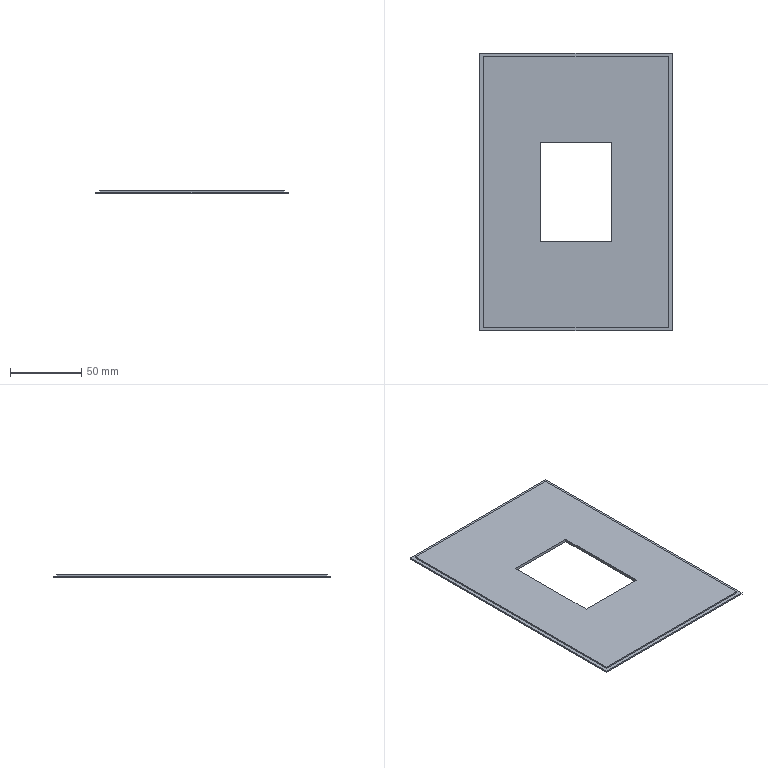Part | NX | 1 solid | 15 faces | box 135 x 195 x 2 mm | volume 44025 mm3 | plane 15
STEP:
#1=CARTESIAN_POINT('',(67.5,-97.5,1.));
#2=VERTEX_POINT('',#1);
#3=CARTESIAN_POINT('',(67.5,97.5,1.));
#4=VERTEX_POINT('',#3);
#5=CARTESIAN_POINT('',(67.5,97.5,1.));
#6=DIRECTION('',(0.,1.,0.));
#7=VECTOR('',#6,1000.);
#8=LINE('',#5,#7);
#9=EDGE_CURVE('',#2,#4,#8,.T.);
#10=ORIENTED_EDGE('',*,*,#9,.T.);
#11=CARTESIAN_POINT('',(-67.5,97.5,1.));
#12=VERTEX_POINT('',#11);
#13=CARTESIAN_POINT('',(-67.5,97.5,1.));
#14=DIRECTION('',(-1.,0.,0.));
#15=VECTOR('',#14,1000.);
#16=LINE('',#13,#15);
#17=EDGE_CURVE('',#4,#12,#16,.T.);
#18=ORIENTED_EDGE('',*,*,#17,.T.);
#19=CARTESIAN_POINT('',(-67.5,-97.5,1.));
#20=VERTEX_POINT('',#19);
#21=CARTESIAN_POINT('',(-67.5,97.5,1.));
#22=DIRECTION('',(0.,-1.,0.));
#23=VECTOR('',#22,1000.);
#24=LINE('',#21,#23);
#25=EDGE_CURVE('',#12,#20,#24,.T.);
#26=ORIENTED_EDGE('',*,*,#25,.T.);
#27=CARTESIAN_POINT('',(-67.5,-97.5,1.));
#28=DIRECTION('',(1.,0.,0.));
#29=VECTOR('',#28,1000.);
#30=LINE('',#27,#29);
#31=EDGE_CURVE('',#20,#2,#30,.T.);
#32=ORIENTED_EDGE('',*,*,#31,.T.);
#33=EDGE_LOOP('',(#10,#18,#26,#32));
#34=FACE_BOUND('',#33,.T.);
#35=CARTESIAN_POINT('',(65.,95.,1.));
#36=VERTEX_POINT('',#35);
#37=CARTESIAN_POINT('',(-65.,95.,1.));
#38=VERTEX_POINT('',#37);
#39=CARTESIAN_POINT('',(-65.,95.,1.));
#40=DIRECTION('',(-1.,0.,0.));
#41=VECTOR('',#40,1000.);
#42=LINE('',#39,#41);
#43=EDGE_CURVE('',#36,#38,#42,.T.);
#44=ORIENTED_EDGE('',*,*,#43,.F.);
#45=CARTESIAN_POINT('',(65.,-95.,1.));
#46=VERTEX_POINT('',#45);
#47=CARTESIAN_POINT('',(65.,95.,1.));
#48=DIRECTION('',(0.,1.,0.));
#49=VECTOR('',#48,1000.);
#50=LINE('',#47,#49);
#51=EDGE_CURVE('',#46,#36,#50,.T.);
#52=ORIENTED_EDGE('',*,*,#51,.F.);
#53=CARTESIAN_POINT('',(-65.,-95.,1.));
#54=VERTEX_POINT('',#53);
#55=CARTESIAN_POINT('',(-65.,-95.,1.));
#56=DIRECTION('',(1.,0.,0.));
#57=VECTOR('',#56,1000.);
#58=LINE('',#55,#57);
#59=EDGE_CURVE('',#54,#46,#58,.T.);
#60=ORIENTED_EDGE('',*,*,#59,.F.);
#61=CARTESIAN_POINT('',(-65.,95.,1.));
#62=DIRECTION('',(0.,-1.,0.));
#63=VECTOR('',#62,1000.);
#64=LINE('',#61,#63);
#65=EDGE_CURVE('',#38,#54,#64,.T.);
#66=ORIENTED_EDGE('',*,*,#65,.F.);
#67=EDGE_LOOP('',(#44,#52,#60,#66));
#68=FACE_BOUND('',#67,.T.);
#69=CARTESIAN_POINT('',(0.,0.,1.));
#70=DIRECTION('',(0.,0.,1.));
#71=DIRECTION('',(1.,0.,0.));
#72=AXIS2_PLACEMENT_3D('',#69,#70,#71);
#73=PLANE('',#72);
#74=ADVANCED_FACE('',(#34,#68),#73,.T.);
#75=CARTESIAN_POINT('',(67.5,-97.5,0.));
#76=VERTEX_POINT('',#75);
#77=CARTESIAN_POINT('',(67.5,97.5,0.));
#78=VERTEX_POINT('',#77);
#79=CARTESIAN_POINT('',(67.5,97.5,0.));
#80=DIRECTION('',(0.,1.,0.));
#81=VECTOR('',#80,1000.);
#82=LINE('',#79,#81);
#83=EDGE_CURVE('',#76,#78,#82,.T.);
#84=ORIENTED_EDGE('',*,*,#83,.T.);
#85=CARTESIAN_POINT('',(67.5,97.5,1.));
#86=DIRECTION('',(0.,0.,-1.));
#87=VECTOR('',#86,1000.);
#88=LINE('',#85,#87);
#89=EDGE_CURVE('',#4,#78,#88,.T.);
#90=ORIENTED_EDGE('',*,*,#89,.F.);
#91=ORIENTED_EDGE('',*,*,#9,.F.);
#92=CARTESIAN_POINT('',(67.5,-97.5,1.));
#93=DIRECTION('',(0.,0.,-1.));
#94=VECTOR('',#93,1000.);
#95=LINE('',#92,#94);
#96=EDGE_CURVE('',#2,#76,#95,.T.);
#97=ORIENTED_EDGE('',*,*,#96,.T.);
#98=EDGE_LOOP('',(#84,#90,#91,#97));
#99=FACE_BOUND('',#98,.T.);
#100=CARTESIAN_POINT('',(67.5,97.5,1.));
#101=DIRECTION('',(-1.,0.,0.));
#102=DIRECTION('',(0.,-1.,0.));
#103=AXIS2_PLACEMENT_3D('',#100,#101,#102);
#104=PLANE('',#103);
#105=ADVANCED_FACE('',(#99),#104,.F.);
#106=CARTESIAN_POINT('',(-67.5,97.5,0.));
#107=VERTEX_POINT('',#106);
#108=CARTESIAN_POINT('',(-67.5,97.5,0.));
#109=DIRECTION('',(-1.,0.,0.));
#110=VECTOR('',#109,1000.);
#111=LINE('',#108,#110);
#112=EDGE_CURVE('',#78,#107,#111,.T.);
#113=ORIENTED_EDGE('',*,*,#112,.T.);
#114=CARTESIAN_POINT('',(-67.5,97.5,1.));
#115=DIRECTION('',(0.,0.,-1.));
#116=VECTOR('',#115,1000.);
#117=LINE('',#114,#116);
#118=EDGE_CURVE('',#12,#107,#117,.T.);
#119=ORIENTED_EDGE('',*,*,#118,.F.);
#120=ORIENTED_EDGE('',*,*,#17,.F.);
#121=ORIENTED_EDGE('',*,*,#89,.T.);
#122=EDGE_LOOP('',(#113,#119,#120,#121));
#123=FACE_BOUND('',#122,.T.);
#124=CARTESIAN_POINT('',(-67.5,97.5,1.));
#125=DIRECTION('',(0.,-1.,0.));
#126=DIRECTION('',(0.,0.,-1.));
#127=AXIS2_PLACEMENT_3D('',#124,#125,#126);
#128=PLANE('',#127);
#129=ADVANCED_FACE('',(#123),#128,.F.);
#130=CARTESIAN_POINT('',(-67.5,-97.5,0.));
#131=VERTEX_POINT('',#130);
#132=CARTESIAN_POINT('',(-67.5,97.5,0.));
#133=DIRECTION('',(0.,-1.,0.));
#134=VECTOR('',#133,1000.);
#135=LINE('',#132,#134);
#136=EDGE_CURVE('',#107,#131,#135,.T.);
#137=ORIENTED_EDGE('',*,*,#136,.T.);
#138=CARTESIAN_POINT('',(-67.5,-97.5,1.));
#139=DIRECTION('',(0.,0.,-1.));
#140=VECTOR('',#139,1000.);
#141=LINE('',#138,#140);
#142=EDGE_CURVE('',#20,#131,#141,.T.);
#143=ORIENTED_EDGE('',*,*,#142,.F.);
#144=ORIENTED_EDGE('',*,*,#25,.F.);
#145=ORIENTED_EDGE('',*,*,#118,.T.);
#146=EDGE_LOOP('',(#137,#143,#144,#145));
#147=FACE_BOUND('',#146,.T.);
#148=CARTESIAN_POINT('',(-67.5,97.5,1.));
#149=DIRECTION('',(1.,0.,0.));
#150=DIRECTION('',(0.,1.,0.));
#151=AXIS2_PLACEMENT_3D('',#148,#149,#150);
#152=PLANE('',#151);
#153=ADVANCED_FACE('',(#147),#152,.F.);
#154=CARTESIAN_POINT('',(-67.5,-97.5,0.));
#155=DIRECTION('',(1.,0.,0.));
#156=VECTOR('',#155,1000.);
#157=LINE('',#154,#156);
#158=EDGE_CURVE('',#131,#76,#157,.T.);
#159=ORIENTED_EDGE('',*,*,#158,.T.);
#160=ORIENTED_EDGE('',*,*,#96,.F.);
#161=ORIENTED_EDGE('',*,*,#31,.F.);
#162=ORIENTED_EDGE('',*,*,#142,.T.);
#163=EDGE_LOOP('',(#159,#160,#161,#162));
#164=FACE_BOUND('',#163,.T.);
#165=CARTESIAN_POINT('',(-67.5,-97.5,1.));
#166=DIRECTION('',(0.,1.,0.));
#167=DIRECTION('',(0.,0.,1.));
#168=AXIS2_PLACEMENT_3D('',#165,#166,#167);
#169=PLANE('',#168);
#170=ADVANCED_FACE('',(#164),#169,.F.);
#171=CARTESIAN_POINT('',(-25.,-35.,0.));
#172=VERTEX_POINT('',#171);
#173=CARTESIAN_POINT('',(25.,-35.,0.));
#174=VERTEX_POINT('',#173);
#175=CARTESIAN_POINT('',(0.,-35.,0.));
#176=DIRECTION('',(1.,0.,0.));
#177=VECTOR('',#176,1000.);
#178=LINE('',#175,#177);
#179=EDGE_CURVE('',#172,#174,#178,.T.);
#180=ORIENTED_EDGE('',*,*,#179,.T.);
#181=CARTESIAN_POINT('',(25.,35.,0.));
#182=VERTEX_POINT('',#181);
#183=CARTESIAN_POINT('',(25.,0.,0.));
#184=DIRECTION('',(0.,1.,0.));
#185=VECTOR('',#184,1000.);
#186=LINE('',#183,#185);
#187=EDGE_CURVE('',#174,#182,#186,.T.);
#188=ORIENTED_EDGE('',*,*,#187,.T.);
#189=CARTESIAN_POINT('',(-25.,35.,0.));
#190=VERTEX_POINT('',#189);
#191=CARTESIAN_POINT('',(0.,35.,0.));
#192=DIRECTION('',(-1.,0.,0.));
#193=VECTOR('',#192,1000.);
#194=LINE('',#191,#193);
#195=EDGE_CURVE('',#182,#190,#194,.T.);
#196=ORIENTED_EDGE('',*,*,#195,.T.);
#197=CARTESIAN_POINT('',(-25.,0.,0.));
#198=DIRECTION('',(0.,-1.,0.));
#199=VECTOR('',#198,1000.);
#200=LINE('',#197,#199);
#201=EDGE_CURVE('',#190,#172,#200,.T.);
#202=ORIENTED_EDGE('',*,*,#201,.T.);
#203=EDGE_LOOP('',(#180,#188,#196,#202));
#204=FACE_BOUND('',#203,.T.);
#205=ORIENTED_EDGE('',*,*,#83,.F.);
#206=ORIENTED_EDGE('',*,*,#158,.F.);
#207=ORIENTED_EDGE('',*,*,#136,.F.);
#208=ORIENTED_EDGE('',*,*,#112,.F.);
#209=EDGE_LOOP('',(#205,#206,#207,#208));
#210=FACE_BOUND('',#209,.T.);
#211=CARTESIAN_POINT('',(0.,0.,0.));
#212=DIRECTION('',(0.,0.,1.));
#213=DIRECTION('',(1.,0.,0.));
#214=AXIS2_PLACEMENT_3D('',#211,#212,#213);
#215=PLANE('',#214);
#216=ADVANCED_FACE('',(#204,#210),#215,.F.);
#217=ORIENTED_EDGE('',*,*,#51,.T.);
#218=CARTESIAN_POINT('',(65.,95.,2.));
#219=VERTEX_POINT('',#218);
#220=CARTESIAN_POINT('',(65.,95.,2.));
#221=DIRECTION('',(0.,0.,-1.));
#222=VECTOR('',#221,1000.);
#223=LINE('',#220,#222);
#224=EDGE_CURVE('',#219,#36,#223,.T.);
#225=ORIENTED_EDGE('',*,*,#224,.F.);
#226=CARTESIAN_POINT('',(65.,-95.,2.));
#227=VERTEX_POINT('',#226);
#228=CARTESIAN_POINT('',(65.,95.,2.));
#229=DIRECTION('',(0.,1.,0.));
#230=VECTOR('',#229,1000.);
#231=LINE('',#228,#230);
#232=EDGE_CURVE('',#227,#219,#231,.T.);
#233=ORIENTED_EDGE('',*,*,#232,.F.);
#234=CARTESIAN_POINT('',(65.,-95.,2.));
#235=DIRECTION('',(0.,0.,-1.));
#236=VECTOR('',#235,1000.);
#237=LINE('',#234,#236);
#238=EDGE_CURVE('',#227,#46,#237,.T.);
#239=ORIENTED_EDGE('',*,*,#238,.T.);
#240=EDGE_LOOP('',(#217,#225,#233,#239));
#241=FACE_BOUND('',#240,.T.);
#242=CARTESIAN_POINT('',(65.,95.,2.));
#243=DIRECTION('',(-1.,0.,0.));
#244=DIRECTION('',(0.,-1.,0.));
#245=AXIS2_PLACEMENT_3D('',#242,#243,#244);
#246=PLANE('',#245);
#247=ADVANCED_FACE('',(#241),#246,.F.);
#248=ORIENTED_EDGE('',*,*,#43,.T.);
#249=CARTESIAN_POINT('',(-65.,95.,2.));
#250=VERTEX_POINT('',#249);
#251=CARTESIAN_POINT('',(-65.,95.,2.));
#252=DIRECTION('',(0.,0.,-1.));
#253=VECTOR('',#252,1000.);
#254=LINE('',#251,#253);
#255=EDGE_CURVE('',#250,#38,#254,.T.);
#256=ORIENTED_EDGE('',*,*,#255,.F.);
#257=CARTESIAN_POINT('',(-65.,95.,2.));
#258=DIRECTION('',(-1.,0.,0.));
#259=VECTOR('',#258,1000.);
#260=LINE('',#257,#259);
#261=EDGE_CURVE('',#219,#250,#260,.T.);
#262=ORIENTED_EDGE('',*,*,#261,.F.);
#263=ORIENTED_EDGE('',*,*,#224,.T.);
#264=EDGE_LOOP('',(#248,#256,#262,#263));
#265=FACE_BOUND('',#264,.T.);
#266=CARTESIAN_POINT('',(-65.,95.,2.));
#267=DIRECTION('',(0.,-1.,0.));
#268=DIRECTION('',(0.,0.,-1.));
#269=AXIS2_PLACEMENT_3D('',#266,#267,#268);
#270=PLANE('',#269);
#271=ADVANCED_FACE('',(#265),#270,.F.);
#272=ORIENTED_EDGE('',*,*,#65,.T.);
#273=CARTESIAN_POINT('',(-65.,-95.,2.));
#274=VERTEX_POINT('',#273);
#275=CARTESIAN_POINT('',(-65.,-95.,2.));
#276=DIRECTION('',(0.,0.,-1.));
#277=VECTOR('',#276,1000.);
#278=LINE('',#275,#277);
#279=EDGE_CURVE('',#274,#54,#278,.T.);
#280=ORIENTED_EDGE('',*,*,#279,.F.);
#281=CARTESIAN_POINT('',(-65.,95.,2.));
#282=DIRECTION('',(0.,-1.,0.));
#283=VECTOR('',#282,1000.);
#284=LINE('',#281,#283);
#285=EDGE_CURVE('',#250,#274,#284,.T.);
#286=ORIENTED_EDGE('',*,*,#285,.F.);
#287=ORIENTED_EDGE('',*,*,#255,.T.);
#288=EDGE_LOOP('',(#272,#280,#286,#287));
#289=FACE_BOUND('',#288,.T.);
#290=CARTESIAN_POINT('',(-65.,95.,2.));
#291=DIRECTION('',(1.,0.,0.));
#292=DIRECTION('',(0.,1.,0.));
#293=AXIS2_PLACEMENT_3D('',#290,#291,#292);
#294=PLANE('',#293);
#295=ADVANCED_FACE('',(#289),#294,.F.);
#296=ORIENTED_EDGE('',*,*,#59,.T.);
#297=ORIENTED_EDGE('',*,*,#238,.F.);
#298=CARTESIAN_POINT('',(-65.,-95.,2.));
#299=DIRECTION('',(1.,0.,0.));
#300=VECTOR('',#299,1000.);
#301=LINE('',#298,#300);
#302=EDGE_CURVE('',#274,#227,#301,.T.);
#303=ORIENTED_EDGE('',*,*,#302,.F.);
#304=ORIENTED_EDGE('',*,*,#279,.T.);
#305=EDGE_LOOP('',(#296,#297,#303,#304));
#306=FACE_BOUND('',#305,.T.);
#307=CARTESIAN_POINT('',(-65.,-95.,2.));
#308=DIRECTION('',(0.,1.,0.));
#309=DIRECTION('',(0.,0.,1.));
#310=AXIS2_PLACEMENT_3D('',#307,#308,#309);
#311=PLANE('',#310);
#312=ADVANCED_FACE('',(#306),#311,.F.);
#313=CARTESIAN_POINT('',(25.,-35.,2.));
#314=VERTEX_POINT('',#313);
#315=CARTESIAN_POINT('',(25.,35.,2.));
#316=VERTEX_POINT('',#315);
#317=CARTESIAN_POINT('',(25.,35.,2.));
#318=DIRECTION('',(0.,1.,0.));
#319=VECTOR('',#318,1000.);
#320=LINE('',#317,#319);
#321=EDGE_CURVE('',#314,#316,#320,.T.);
#322=ORIENTED_EDGE('',*,*,#321,.F.);
#323=CARTESIAN_POINT('',(-25.,-35.,2.));
#324=VERTEX_POINT('',#323);
#325=CARTESIAN_POINT('',(-25.,-35.,2.));
#326=DIRECTION('',(1.,0.,0.));
#327=VECTOR('',#326,1000.);
#328=LINE('',#325,#327);
#329=EDGE_CURVE('',#324,#314,#328,.T.);
#330=ORIENTED_EDGE('',*,*,#329,.F.);
#331=CARTESIAN_POINT('',(-25.,35.,2.));
#332=VERTEX_POINT('',#331);
#333=CARTESIAN_POINT('',(-25.,35.,2.));
#334=DIRECTION('',(0.,-1.,0.));
#335=VECTOR('',#334,1000.);
#336=LINE('',#333,#335);
#337=EDGE_CURVE('',#332,#324,#336,.T.);
#338=ORIENTED_EDGE('',*,*,#337,.F.);
#339=CARTESIAN_POINT('',(-25.,35.,2.));
#340=DIRECTION('',(-1.,0.,0.));
#341=VECTOR('',#340,1000.);
#342=LINE('',#339,#341);
#343=EDGE_CURVE('',#316,#332,#342,.T.);
#344=ORIENTED_EDGE('',*,*,#343,.F.);
#345=EDGE_LOOP('',(#322,#330,#338,#344));
#346=FACE_BOUND('',#345,.T.);
#347=ORIENTED_EDGE('',*,*,#232,.T.);
#348=ORIENTED_EDGE('',*,*,#261,.T.);
#349=ORIENTED_EDGE('',*,*,#285,.T.);
#350=ORIENTED_EDGE('',*,*,#302,.T.);
#351=EDGE_LOOP('',(#347,#348,#349,#350));
#352=FACE_BOUND('',#351,.T.);
#353=CARTESIAN_POINT('',(0.,0.,2.));
#354=DIRECTION('',(0.,0.,1.));
#355=DIRECTION('',(1.,0.,0.));
#356=AXIS2_PLACEMENT_3D('',#353,#354,#355);
#357=PLANE('',#356);
#358=ADVANCED_FACE('',(#346,#352),#357,.T.);
#359=CARTESIAN_POINT('',(25.,-35.,-1.));
#360=DIRECTION('',(0.,0.,1.));
#361=VECTOR('',#360,1000.);
#362=LINE('',#359,#361);
#363=EDGE_CURVE('',#174,#314,#362,.T.);
#364=ORIENTED_EDGE('',*,*,#363,.T.);
#365=ORIENTED_EDGE('',*,*,#321,.T.);
#366=CARTESIAN_POINT('',(25.,35.,-1.));
#367=DIRECTION('',(0.,0.,1.));
#368=VECTOR('',#367,1000.);
#369=LINE('',#366,#368);
#370=EDGE_CURVE('',#182,#316,#369,.T.);
#371=ORIENTED_EDGE('',*,*,#370,.F.);
#372=ORIENTED_EDGE('',*,*,#187,.F.);
#373=EDGE_LOOP('',(#364,#365,#371,#372));
#374=FACE_BOUND('',#373,.T.);
#375=CARTESIAN_POINT('',(25.,35.,-1.));
#376=DIRECTION('',(1.,0.,0.));
#377=DIRECTION('',(0.,1.,0.));
#378=AXIS2_PLACEMENT_3D('',#375,#376,#377);
#379=PLANE('',#378);
#380=ADVANCED_FACE('',(#374),#379,.F.);
#381=CARTESIAN_POINT('',(-25.,-35.,-1.));
#382=DIRECTION('',(0.,0.,1.));
#383=VECTOR('',#382,1000.);
#384=LINE('',#381,#383);
#385=EDGE_CURVE('',#172,#324,#384,.T.);
#386=ORIENTED_EDGE('',*,*,#385,.T.);
#387=ORIENTED_EDGE('',*,*,#329,.T.);
#388=ORIENTED_EDGE('',*,*,#363,.F.);
#389=ORIENTED_EDGE('',*,*,#179,.F.);
#390=EDGE_LOOP('',(#386,#387,#388,#389));
#391=FACE_BOUND('',#390,.T.);
#392=CARTESIAN_POINT('',(-25.,-35.,-1.));
#393=DIRECTION('',(0.,-1.,0.));
#394=DIRECTION('',(0.,0.,-1.));
#395=AXIS2_PLACEMENT_3D('',#392,#393,#394);
#396=PLANE('',#395);
#397=ADVANCED_FACE('',(#391),#396,.F.);
#398=CARTESIAN_POINT('',(-25.,35.,-1.));
#399=DIRECTION('',(0.,0.,1.));
#400=VECTOR('',#399,1000.);
#401=LINE('',#398,#400);
#402=EDGE_CURVE('',#190,#332,#401,.T.);
#403=ORIENTED_EDGE('',*,*,#402,.T.);
#404=ORIENTED_EDGE('',*,*,#337,.T.);
#405=ORIENTED_EDGE('',*,*,#385,.F.);
#406=ORIENTED_EDGE('',*,*,#201,.F.);
#407=EDGE_LOOP('',(#403,#404,#405,#406));
#408=FACE_BOUND('',#407,.T.);
#409=CARTESIAN_POINT('',(-25.,35.,-1.));
#410=DIRECTION('',(-1.,0.,0.));
#411=DIRECTION('',(0.,-1.,0.));
#412=AXIS2_PLACEMENT_3D('',#409,#410,#411);
#413=PLANE('',#412);
#414=ADVANCED_FACE('',(#408),#413,.F.);
#415=ORIENTED_EDGE('',*,*,#370,.T.);
#416=ORIENTED_EDGE('',*,*,#343,.T.);
#417=ORIENTED_EDGE('',*,*,#402,.F.);
#418=ORIENTED_EDGE('',*,*,#195,.F.);
#419=EDGE_LOOP('',(#415,#416,#417,#418));
#420=FACE_BOUND('',#419,.T.);
#421=CARTESIAN_POINT('',(-25.,35.,-1.));
#422=DIRECTION('',(0.,1.,0.));
#423=DIRECTION('',(0.,0.,1.));
#424=AXIS2_PLACEMENT_3D('',#421,#422,#423);
#425=PLANE('',#424);
#426=ADVANCED_FACE('',(#420),#425,.F.);
#427=CLOSED_SHELL('',(#74,#105,#129,#153,#170,#216,#247,#271,#295,#312,#358,#380,#397,#414,#426));
#428=MANIFOLD_SOLID_BREP('',#427);
#429=(LENGTH_UNIT()NAMED_UNIT(*)SI_UNIT(.MILLI.,.METRE.));
#430=UNCERTAINTY_MEASURE_WITH_UNIT(LENGTH_MEASURE(0.00001),#429,'','');
#431=(NAMED_UNIT(*)PLANE_ANGLE_UNIT()SI_UNIT($,.RADIAN.));
#432=(NAMED_UNIT(*)SI_UNIT($,.STERADIAN.)SOLID_ANGLE_UNIT());
#433=(GEOMETRIC_REPRESENTATION_CONTEXT(3)GLOBAL_UNCERTAINTY_ASSIGNED_CONTEXT((#430))GLOBAL_UNIT_ASSIGNED_CONTEXT((#429,#431,#432))REPRESENTATION_CONTEXT('',''));
#434=ADVANCED_BREP_SHAPE_REPRESENTATION('',(#428),#433);